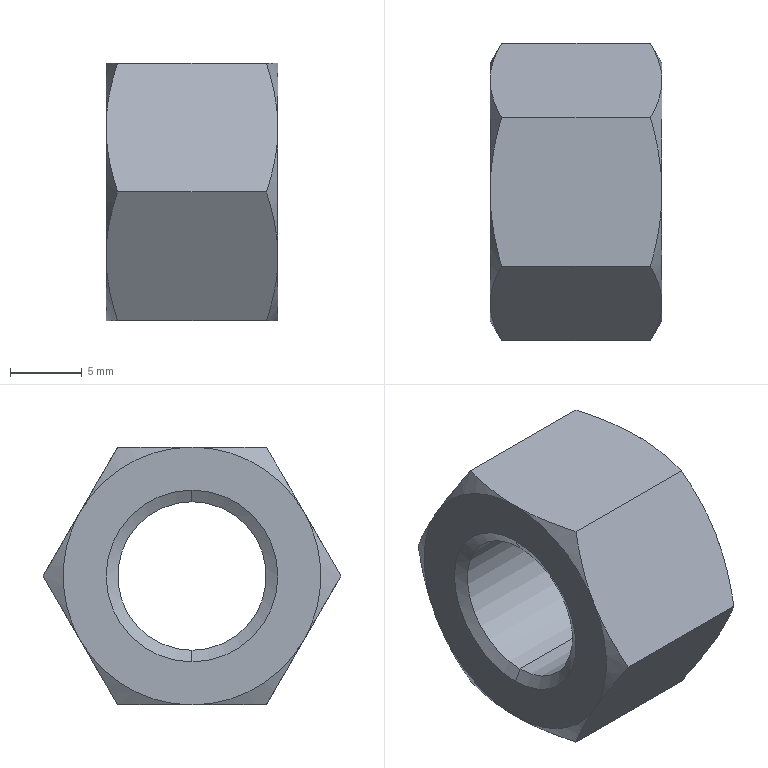Part | SolidWorks | features BaseBody 1 | 1 solid | 26 faces | box 12 x 20.785 x 18 mm | volume 2327 mm3 | cone 16 | plane 8 | cylinder 2 | commonest cylinder face diameters 10.376 x2
STEP:
#1=CARTESIAN_POINT('',(0.4688,0.,5.188));
#2=VERTEX_POINT('',#1);
#3=CARTESIAN_POINT('',(0.4688,0.,-5.188));
#4=VERTEX_POINT('',#3);
#5=CARTESIAN_POINT('',(0.4688,0.,0.));
#6=DIRECTION('',(1.,0.,0.));
#7=DIRECTION('',(0.,0.,-1.));
#8=AXIS2_PLACEMENT_3D('',#5,#6,#7);
#9=CIRCLE('',#8,5.188);
#10=EDGE_CURVE('',#2,#4,#9,.T.);
#11=ORIENTED_EDGE('',*,*,#10,.F.);
#12=CARTESIAN_POINT('',(11.531,0.,5.188));
#13=VERTEX_POINT('',#12);
#14=CARTESIAN_POINT('',(-18.,0.,5.188));
#15=DIRECTION('',(1.,0.,0.));
#16=VECTOR('',#15,1000.);
#17=LINE('',#14,#16);
#18=EDGE_CURVE('',#2,#13,#17,.T.);
#19=ORIENTED_EDGE('',*,*,#18,.T.);
#20=CARTESIAN_POINT('',(11.531,0.,-5.188));
#21=VERTEX_POINT('',#20);
#22=CARTESIAN_POINT('',(11.531,0.,0.));
#23=DIRECTION('',(-1.,0.,0.));
#24=DIRECTION('',(0.,0.,-1.));
#25=AXIS2_PLACEMENT_3D('',#22,#23,#24);
#26=CIRCLE('',#25,5.188);
#27=EDGE_CURVE('',#21,#13,#26,.T.);
#28=ORIENTED_EDGE('',*,*,#27,.F.);
#29=CARTESIAN_POINT('',(-18.,0.,-5.188));
#30=DIRECTION('',(1.,0.,0.));
#31=VECTOR('',#30,1000.);
#32=LINE('',#29,#31);
#33=EDGE_CURVE('',#4,#21,#32,.T.);
#34=ORIENTED_EDGE('',*,*,#33,.F.);
#35=EDGE_LOOP('',(#11,#19,#28,#34));
#36=FACE_OUTER_BOUND('',#35,.T.);
#37=CARTESIAN_POINT('',(-18.,0.,0.));
#38=DIRECTION('',(1.,0.,0.));
#39=DIRECTION('',(0.,0.,-1.));
#40=AXIS2_PLACEMENT_3D('',#37,#38,#39);
#41=CYLINDRICAL_SURFACE('',#40,5.188);
#42=ADVANCED_FACE('',(#36),#41,.F.);
#43=ORIENTED_EDGE('',*,*,#10,.T.);
#44=CARTESIAN_POINT('',(0.,0.,-6.));
#45=VERTEX_POINT('',#44);
#46=CARTESIAN_POINT('',(0.,0.,-6.));
#47=DIRECTION('',(-0.5,0.,-0.866));
#48=VECTOR('',#47,1000.);
#49=LINE('',#46,#48);
#50=EDGE_CURVE('',#4,#45,#49,.T.);
#51=ORIENTED_EDGE('',*,*,#50,.T.);
#52=CARTESIAN_POINT('',(0.,0.,6.));
#53=VERTEX_POINT('',#52);
#54=CARTESIAN_POINT('',(0.,0.,0.));
#55=DIRECTION('',(1.,0.,0.));
#56=DIRECTION('',(0.,0.,1.));
#57=AXIS2_PLACEMENT_3D('',#54,#55,#56);
#58=CIRCLE('',#57,6.);
#59=EDGE_CURVE('',#53,#45,#58,.T.);
#60=ORIENTED_EDGE('',*,*,#59,.F.);
#61=CARTESIAN_POINT('',(0.,0.,6.));
#62=DIRECTION('',(-0.5,0.,0.866));
#63=VECTOR('',#62,1000.);
#64=LINE('',#61,#63);
#65=EDGE_CURVE('',#2,#53,#64,.T.);
#66=ORIENTED_EDGE('',*,*,#65,.F.);
#67=EDGE_LOOP('',(#43,#51,#60,#66));
#68=FACE_OUTER_BOUND('',#67,.T.);
#69=CARTESIAN_POINT('',(0.,0.,0.));
#70=DIRECTION('',(-1.,0.,0.));
#71=DIRECTION('',(0.,0.,1.));
#72=AXIS2_PLACEMENT_3D('',#69,#70,#71);
#73=CONICAL_SURFACE('',#72,6.,1.047);
#74=ADVANCED_FACE('',(#68),#73,.F.);
#75=ORIENTED_EDGE('',*,*,#27,.T.);
#76=CARTESIAN_POINT('',(12.,0.,6.));
#77=VERTEX_POINT('',#76);
#78=CARTESIAN_POINT('',(12.,0.,6.));
#79=DIRECTION('',(0.5,0.,0.866));
#80=VECTOR('',#79,1000.);
#81=LINE('',#78,#80);
#82=EDGE_CURVE('',#13,#77,#81,.T.);
#83=ORIENTED_EDGE('',*,*,#82,.T.);
#84=CARTESIAN_POINT('',(12.,0.,-6.));
#85=VERTEX_POINT('',#84);
#86=CARTESIAN_POINT('',(12.,0.,0.));
#87=DIRECTION('',(-1.,0.,0.));
#88=DIRECTION('',(0.,0.,-1.));
#89=AXIS2_PLACEMENT_3D('',#86,#87,#88);
#90=CIRCLE('',#89,6.);
#91=EDGE_CURVE('',#85,#77,#90,.T.);
#92=ORIENTED_EDGE('',*,*,#91,.F.);
#93=CARTESIAN_POINT('',(12.,0.,-6.));
#94=DIRECTION('',(0.5,0.,-0.866));
#95=VECTOR('',#94,1000.);
#96=LINE('',#93,#95);
#97=EDGE_CURVE('',#21,#85,#96,.T.);
#98=ORIENTED_EDGE('',*,*,#97,.F.);
#99=EDGE_LOOP('',(#75,#83,#92,#98));
#100=FACE_OUTER_BOUND('',#99,.T.);
#101=CARTESIAN_POINT('',(12.,0.,0.));
#102=DIRECTION('',(1.,0.,0.));
#103=DIRECTION('',(0.,0.,-1.));
#104=AXIS2_PLACEMENT_3D('',#101,#102,#103);
#105=CONICAL_SURFACE('',#104,6.,1.047);
#106=ADVANCED_FACE('',(#100),#105,.F.);
#107=ORIENTED_EDGE('',*,*,#18,.F.);
#108=CARTESIAN_POINT('',(0.4688,0.,0.));
#109=DIRECTION('',(1.,0.,0.));
#110=DIRECTION('',(0.,0.,-1.));
#111=AXIS2_PLACEMENT_3D('',#108,#109,#110);
#112=CIRCLE('',#111,5.188);
#113=EDGE_CURVE('',#4,#2,#112,.T.);
#114=ORIENTED_EDGE('',*,*,#113,.F.);
#115=ORIENTED_EDGE('',*,*,#33,.T.);
#116=CARTESIAN_POINT('',(11.531,0.,0.));
#117=DIRECTION('',(-1.,0.,0.));
#118=DIRECTION('',(0.,0.,-1.));
#119=AXIS2_PLACEMENT_3D('',#116,#117,#118);
#120=CIRCLE('',#119,5.188);
#121=EDGE_CURVE('',#13,#21,#120,.T.);
#122=ORIENTED_EDGE('',*,*,#121,.F.);
#123=EDGE_LOOP('',(#107,#114,#115,#122));
#124=FACE_OUTER_BOUND('',#123,.T.);
#125=CARTESIAN_POINT('',(-18.,0.,0.));
#126=DIRECTION('',(1.,0.,0.));
#127=DIRECTION('',(0.,0.,-1.));
#128=AXIS2_PLACEMENT_3D('',#125,#126,#127);
#129=CYLINDRICAL_SURFACE('',#128,5.188);
#130=ADVANCED_FACE('',(#124),#129,.F.);
#131=ORIENTED_EDGE('',*,*,#50,.F.);
#132=ORIENTED_EDGE('',*,*,#113,.T.);
#133=ORIENTED_EDGE('',*,*,#65,.T.);
#134=CARTESIAN_POINT('',(0.,0.,0.));
#135=DIRECTION('',(1.,0.,0.));
#136=DIRECTION('',(0.,0.,1.));
#137=AXIS2_PLACEMENT_3D('',#134,#135,#136);
#138=CIRCLE('',#137,6.);
#139=EDGE_CURVE('',#45,#53,#138,.T.);
#140=ORIENTED_EDGE('',*,*,#139,.F.);
#141=EDGE_LOOP('',(#131,#132,#133,#140));
#142=FACE_OUTER_BOUND('',#141,.T.);
#143=CARTESIAN_POINT('',(0.,0.,0.));
#144=DIRECTION('',(-1.,0.,0.));
#145=DIRECTION('',(0.,0.,1.));
#146=AXIS2_PLACEMENT_3D('',#143,#144,#145);
#147=CONICAL_SURFACE('',#146,6.,1.047);
#148=ADVANCED_FACE('',(#142),#147,.F.);
#149=ORIENTED_EDGE('',*,*,#82,.F.);
#150=ORIENTED_EDGE('',*,*,#121,.T.);
#151=ORIENTED_EDGE('',*,*,#97,.T.);
#152=CARTESIAN_POINT('',(12.,0.,0.));
#153=DIRECTION('',(-1.,0.,0.));
#154=DIRECTION('',(0.,0.,-1.));
#155=AXIS2_PLACEMENT_3D('',#152,#153,#154);
#156=CIRCLE('',#155,6.);
#157=EDGE_CURVE('',#77,#85,#156,.T.);
#158=ORIENTED_EDGE('',*,*,#157,.F.);
#159=EDGE_LOOP('',(#149,#150,#151,#158));
#160=FACE_OUTER_BOUND('',#159,.T.);
#161=CARTESIAN_POINT('',(12.,0.,0.));
#162=DIRECTION('',(1.,0.,0.));
#163=DIRECTION('',(0.,0.,-1.));
#164=AXIS2_PLACEMENT_3D('',#161,#162,#163);
#165=CONICAL_SURFACE('',#164,6.,1.047);
#166=ADVANCED_FACE('',(#160),#165,.F.);
#167=ORIENTED_EDGE('',*,*,#59,.T.);
#168=ORIENTED_EDGE('',*,*,#139,.T.);
#169=EDGE_LOOP('',(#167,#168));
#170=FACE_BOUND('',#169,.T.);
#171=CARTESIAN_POINT('',(0.,0.,9.));
#172=VERTEX_POINT('',#171);
#173=CARTESIAN_POINT('',(0.,-7.794,4.5));
#174=VERTEX_POINT('',#173);
#175=CARTESIAN_POINT('',(0.,0.,0.));
#176=DIRECTION('',(1.,0.,0.));
#177=DIRECTION('',(0.,0.,-1.));
#178=AXIS2_PLACEMENT_3D('',#175,#176,#177);
#179=CIRCLE('',#178,9.);
#180=EDGE_CURVE('',#172,#174,#179,.T.);
#181=ORIENTED_EDGE('',*,*,#180,.F.);
#182=CARTESIAN_POINT('',(0.,7.794,4.5));
#183=VERTEX_POINT('',#182);
#184=CARTESIAN_POINT('',(0.,0.,0.));
#185=DIRECTION('',(1.,0.,0.));
#186=DIRECTION('',(0.,0.,-1.));
#187=AXIS2_PLACEMENT_3D('',#184,#185,#186);
#188=CIRCLE('',#187,9.);
#189=EDGE_CURVE('',#183,#172,#188,.T.);
#190=ORIENTED_EDGE('',*,*,#189,.F.);
#191=CARTESIAN_POINT('',(0.,7.794,-4.5));
#192=VERTEX_POINT('',#191);
#193=CARTESIAN_POINT('',(0.,0.,0.));
#194=DIRECTION('',(1.,0.,0.));
#195=DIRECTION('',(0.,0.,-1.));
#196=AXIS2_PLACEMENT_3D('',#193,#194,#195);
#197=CIRCLE('',#196,9.);
#198=EDGE_CURVE('',#192,#183,#197,.T.);
#199=ORIENTED_EDGE('',*,*,#198,.F.);
#200=CARTESIAN_POINT('',(0.,0.,-9.));
#201=VERTEX_POINT('',#200);
#202=CARTESIAN_POINT('',(0.,0.,0.));
#203=DIRECTION('',(1.,0.,0.));
#204=DIRECTION('',(0.,0.,-1.));
#205=AXIS2_PLACEMENT_3D('',#202,#203,#204);
#206=CIRCLE('',#205,9.);
#207=EDGE_CURVE('',#201,#192,#206,.T.);
#208=ORIENTED_EDGE('',*,*,#207,.F.);
#209=CARTESIAN_POINT('',(0.,-7.794,-4.5));
#210=VERTEX_POINT('',#209);
#211=CARTESIAN_POINT('',(0.,0.,0.));
#212=DIRECTION('',(1.,0.,0.));
#213=DIRECTION('',(0.,0.,-1.));
#214=AXIS2_PLACEMENT_3D('',#211,#212,#213);
#215=CIRCLE('',#214,9.);
#216=EDGE_CURVE('',#210,#201,#215,.T.);
#217=ORIENTED_EDGE('',*,*,#216,.F.);
#218=CARTESIAN_POINT('',(0.,0.,0.));
#219=DIRECTION('',(1.,0.,0.));
#220=DIRECTION('',(0.,0.,-1.));
#221=AXIS2_PLACEMENT_3D('',#218,#219,#220);
#222=CIRCLE('',#221,9.);
#223=EDGE_CURVE('',#174,#210,#222,.T.);
#224=ORIENTED_EDGE('',*,*,#223,.F.);
#225=EDGE_LOOP('',(#181,#190,#199,#208,#217,#224));
#226=FACE_OUTER_BOUND('',#225,.T.);
#227=CARTESIAN_POINT('',(0.,0.,0.));
#228=DIRECTION('',(1.,0.,0.));
#229=DIRECTION('',(0.,0.,-1.));
#230=AXIS2_PLACEMENT_3D('',#227,#228,#229);
#231=PLANE('',#230);
#232=ADVANCED_FACE('',(#170,#226),#231,.F.);
#233=ORIENTED_EDGE('',*,*,#91,.T.);
#234=ORIENTED_EDGE('',*,*,#157,.T.);
#235=EDGE_LOOP('',(#233,#234));
#236=FACE_BOUND('',#235,.T.);
#237=CARTESIAN_POINT('',(12.,0.,9.));
#238=VERTEX_POINT('',#237);
#239=CARTESIAN_POINT('',(12.,-7.794,4.5));
#240=VERTEX_POINT('',#239);
#241=CARTESIAN_POINT('',(12.,0.,0.));
#242=DIRECTION('',(1.,0.,0.));
#243=DIRECTION('',(0.,0.,1.));
#244=AXIS2_PLACEMENT_3D('',#241,#242,#243);
#245=CIRCLE('',#244,9.);
#246=EDGE_CURVE('',#238,#240,#245,.T.);
#247=ORIENTED_EDGE('',*,*,#246,.T.);
#248=CARTESIAN_POINT('',(12.,-7.794,-4.5));
#249=VERTEX_POINT('',#248);
#250=CARTESIAN_POINT('',(12.,0.,0.));
#251=DIRECTION('',(1.,0.,0.));
#252=DIRECTION('',(0.,0.,1.));
#253=AXIS2_PLACEMENT_3D('',#250,#251,#252);
#254=CIRCLE('',#253,9.);
#255=EDGE_CURVE('',#240,#249,#254,.T.);
#256=ORIENTED_EDGE('',*,*,#255,.T.);
#257=CARTESIAN_POINT('',(12.,0.,-9.));
#258=VERTEX_POINT('',#257);
#259=CARTESIAN_POINT('',(12.,0.,0.));
#260=DIRECTION('',(1.,0.,0.));
#261=DIRECTION('',(0.,0.,1.));
#262=AXIS2_PLACEMENT_3D('',#259,#260,#261);
#263=CIRCLE('',#262,9.);
#264=EDGE_CURVE('',#249,#258,#263,.T.);
#265=ORIENTED_EDGE('',*,*,#264,.T.);
#266=CARTESIAN_POINT('',(12.,7.794,-4.5));
#267=VERTEX_POINT('',#266);
#268=CARTESIAN_POINT('',(12.,0.,0.));
#269=DIRECTION('',(1.,0.,0.));
#270=DIRECTION('',(0.,0.,1.));
#271=AXIS2_PLACEMENT_3D('',#268,#269,#270);
#272=CIRCLE('',#271,9.);
#273=EDGE_CURVE('',#258,#267,#272,.T.);
#274=ORIENTED_EDGE('',*,*,#273,.T.);
#275=CARTESIAN_POINT('',(12.,7.794,4.5));
#276=VERTEX_POINT('',#275);
#277=CARTESIAN_POINT('',(12.,0.,0.));
#278=DIRECTION('',(1.,0.,0.));
#279=DIRECTION('',(0.,0.,1.));
#280=AXIS2_PLACEMENT_3D('',#277,#278,#279);
#281=CIRCLE('',#280,9.);
#282=EDGE_CURVE('',#267,#276,#281,.T.);
#283=ORIENTED_EDGE('',*,*,#282,.T.);
#284=CARTESIAN_POINT('',(12.,0.,0.));
#285=DIRECTION('',(1.,0.,0.));
#286=DIRECTION('',(0.,0.,1.));
#287=AXIS2_PLACEMENT_3D('',#284,#285,#286);
#288=CIRCLE('',#287,9.);
#289=EDGE_CURVE('',#276,#238,#288,.T.);
#290=ORIENTED_EDGE('',*,*,#289,.T.);
#291=EDGE_LOOP('',(#247,#256,#265,#274,#283,#290));
#292=FACE_OUTER_BOUND('',#291,.T.);
#293=CARTESIAN_POINT('',(12.,0.,0.));
#294=DIRECTION('',(1.,0.,0.));
#295=DIRECTION('',(0.,0.,-1.));
#296=AXIS2_PLACEMENT_3D('',#293,#294,#295);
#297=PLANE('',#296);
#298=ADVANCED_FACE('',(#236,#292),#297,.T.);
#299=ORIENTED_EDGE('',*,*,#223,.T.);
#300=CARTESIAN_POINT('',(0.8038,-10.392,0.000000014));
#301=VERTEX_POINT('',#300);
#302=CARTESIAN_POINT('',(0.,-7.794,-4.5));
#303=CARTESIAN_POINT('',(0.,-8.238,-3.732));
#304=CARTESIAN_POINT('',(0.07685,-8.675,-2.974));
#305=CARTESIAN_POINT('',(0.3567,-9.54,-1.476));
#306=CARTESIAN_POINT('',(0.5588,-9.968,-0.7351));
#307=CARTESIAN_POINT('',(0.8038,-10.392,0.000000014));
#308=B_SPLINE_CURVE_WITH_KNOTS('',3,(#302,#303,#304,#305,#306,#307),.UNSPECIFIED.,.F.,.F.,(4,2,4),(0.,0.002629,0.005258),.UNSPECIFIED.);
#309=EDGE_CURVE('',#210,#301,#308,.T.);
#310=ORIENTED_EDGE('',*,*,#309,.T.);
#311=CARTESIAN_POINT('',(0.8038,-10.392,0.000000014));
#312=CARTESIAN_POINT('',(0.5588,-9.968,0.7351));
#313=CARTESIAN_POINT('',(0.3567,-9.54,1.476));
#314=CARTESIAN_POINT('',(0.07685,-8.675,2.974));
#315=CARTESIAN_POINT('',(0.,-8.238,3.732));
#316=CARTESIAN_POINT('',(0.,-7.794,4.5));
#317=B_SPLINE_CURVE_WITH_KNOTS('',3,(#311,#312,#313,#314,#315,#316),.UNSPECIFIED.,.F.,.F.,(4,2,4),(0.,0.002629,0.005258),.UNSPECIFIED.);
#318=EDGE_CURVE('',#301,#174,#317,.T.);
#319=ORIENTED_EDGE('',*,*,#318,.T.);
#320=EDGE_LOOP('',(#299,#310,#319));
#321=FACE_OUTER_BOUND('',#320,.T.);
#322=CARTESIAN_POINT('',(0.8087,0.,0.));
#323=DIRECTION('',(1.,0.,0.));
#324=DIRECTION('',(0.,0.,-1.));
#325=AXIS2_PLACEMENT_3D('',#322,#323,#324);
#326=CONICAL_SURFACE('',#325,10.401,1.047);
#327=ADVANCED_FACE('',(#321),#326,.T.);
#328=ORIENTED_EDGE('',*,*,#180,.T.);
#329=CARTESIAN_POINT('',(0.8038,-5.196,9.));
#330=VERTEX_POINT('',#329);
#331=CARTESIAN_POINT('',(0.,-7.794,4.5));
#332=CARTESIAN_POINT('',(0.,-7.351,5.268));
#333=CARTESIAN_POINT('',(0.07685,-6.913,6.026));
#334=CARTESIAN_POINT('',(0.3567,-6.048,7.524));
#335=CARTESIAN_POINT('',(0.5588,-5.621,8.265));
#336=CARTESIAN_POINT('',(0.8038,-5.196,9.));
#337=B_SPLINE_CURVE_WITH_KNOTS('',3,(#331,#332,#333,#334,#335,#336),.UNSPECIFIED.,.F.,.F.,(4,2,4),(0.,0.002629,0.005258),.UNSPECIFIED.);
#338=EDGE_CURVE('',#174,#330,#337,.T.);
#339=ORIENTED_EDGE('',*,*,#338,.T.);
#340=CARTESIAN_POINT('',(0.8038,-5.196,9.));
#341=CARTESIAN_POINT('',(0.5588,-4.347,9.));
#342=CARTESIAN_POINT('',(0.3567,-3.492,9.));
#343=CARTESIAN_POINT('',(0.07685,-1.762,9.));
#344=CARTESIAN_POINT('',(0.,-0.8868,9.));
#345=CARTESIAN_POINT('',(0.,0.,9.));
#346=B_SPLINE_CURVE_WITH_KNOTS('',3,(#340,#341,#342,#343,#344,#345),.UNSPECIFIED.,.F.,.F.,(4,2,4),(0.,0.002629,0.005258),.UNSPECIFIED.);
#347=EDGE_CURVE('',#330,#172,#346,.T.);
#348=ORIENTED_EDGE('',*,*,#347,.T.);
#349=EDGE_LOOP('',(#328,#339,#348));
#350=FACE_OUTER_BOUND('',#349,.T.);
#351=CARTESIAN_POINT('',(0.8087,0.,0.));
#352=DIRECTION('',(1.,0.,0.));
#353=DIRECTION('',(0.,0.,-1.));
#354=AXIS2_PLACEMENT_3D('',#351,#352,#353);
#355=CONICAL_SURFACE('',#354,10.401,1.047);
#356=ADVANCED_FACE('',(#350),#355,.T.);
#357=ORIENTED_EDGE('',*,*,#189,.T.);
#358=CARTESIAN_POINT('',(0.8038,5.196,9.));
#359=VERTEX_POINT('',#358);
#360=CARTESIAN_POINT('',(0.,0.,9.));
#361=CARTESIAN_POINT('',(0.,0.8868,9.));
#362=CARTESIAN_POINT('',(0.07685,1.762,9.));
#363=CARTESIAN_POINT('',(0.3567,3.492,9.));
#364=CARTESIAN_POINT('',(0.5588,4.347,9.));
#365=CARTESIAN_POINT('',(0.8038,5.196,9.));
#366=B_SPLINE_CURVE_WITH_KNOTS('',3,(#360,#361,#362,#363,#364,#365),.UNSPECIFIED.,.F.,.F.,(4,2,4),(0.,0.002629,0.005258),.UNSPECIFIED.);
#367=EDGE_CURVE('',#172,#359,#366,.T.);
#368=ORIENTED_EDGE('',*,*,#367,.T.);
#369=CARTESIAN_POINT('',(0.8038,5.196,9.));
#370=CARTESIAN_POINT('',(0.5588,5.621,8.265));
#371=CARTESIAN_POINT('',(0.3567,6.048,7.524));
#372=CARTESIAN_POINT('',(0.07685,6.913,6.026));
#373=CARTESIAN_POINT('',(0.,7.351,5.268));
#374=CARTESIAN_POINT('',(0.,7.794,4.5));
#375=B_SPLINE_CURVE_WITH_KNOTS('',3,(#369,#370,#371,#372,#373,#374),.UNSPECIFIED.,.F.,.F.,(4,2,4),(0.,0.002629,0.005258),.UNSPECIFIED.);
#376=EDGE_CURVE('',#359,#183,#375,.T.);
#377=ORIENTED_EDGE('',*,*,#376,.T.);
#378=EDGE_LOOP('',(#357,#368,#377));
#379=FACE_OUTER_BOUND('',#378,.T.);
#380=CARTESIAN_POINT('',(0.8087,0.,0.));
#381=DIRECTION('',(1.,0.,0.));
#382=DIRECTION('',(0.,0.,-1.));
#383=AXIS2_PLACEMENT_3D('',#380,#381,#382);
#384=CONICAL_SURFACE('',#383,10.401,1.047);
#385=ADVANCED_FACE('',(#379),#384,.T.);
#386=ORIENTED_EDGE('',*,*,#198,.T.);
#387=CARTESIAN_POINT('',(0.8038,10.392,-0.000000014));
#388=VERTEX_POINT('',#387);
#389=CARTESIAN_POINT('',(0.,7.794,4.5));
#390=CARTESIAN_POINT('',(0.,8.238,3.732));
#391=CARTESIAN_POINT('',(0.07685,8.675,2.974));
#392=CARTESIAN_POINT('',(0.3567,9.54,1.476));
#393=CARTESIAN_POINT('',(0.5588,9.968,0.7351));
#394=CARTESIAN_POINT('',(0.8038,10.392,-0.000000014));
#395=B_SPLINE_CURVE_WITH_KNOTS('',3,(#389,#390,#391,#392,#393,#394),.UNSPECIFIED.,.F.,.F.,(4,2,4),(0.,0.002629,0.005258),.UNSPECIFIED.);
#396=EDGE_CURVE('',#183,#388,#395,.T.);
#397=ORIENTED_EDGE('',*,*,#396,.T.);
#398=CARTESIAN_POINT('',(0.8038,10.392,-0.000000014));
#399=CARTESIAN_POINT('',(0.5588,9.968,-0.7351));
#400=CARTESIAN_POINT('',(0.3567,9.54,-1.476));
#401=CARTESIAN_POINT('',(0.07685,8.675,-2.974));
#402=CARTESIAN_POINT('',(0.,8.238,-3.732));
#403=CARTESIAN_POINT('',(0.,7.794,-4.5));
#404=B_SPLINE_CURVE_WITH_KNOTS('',3,(#398,#399,#400,#401,#402,#403),.UNSPECIFIED.,.F.,.F.,(4,2,4),(0.,0.002629,0.005258),.UNSPECIFIED.);
#405=EDGE_CURVE('',#388,#192,#404,.T.);
#406=ORIENTED_EDGE('',*,*,#405,.T.);
#407=EDGE_LOOP('',(#386,#397,#406));
#408=FACE_OUTER_BOUND('',#407,.T.);
#409=CARTESIAN_POINT('',(0.8087,0.,0.));
#410=DIRECTION('',(1.,0.,0.));
#411=DIRECTION('',(0.,0.,-1.));
#412=AXIS2_PLACEMENT_3D('',#409,#410,#411);
#413=CONICAL_SURFACE('',#412,10.401,1.047);
#414=ADVANCED_FACE('',(#408),#413,.T.);
#415=CARTESIAN_POINT('',(0.8038,5.196,-9.));
#416=VERTEX_POINT('',#415);
#417=CARTESIAN_POINT('',(0.8038,5.196,-9.));
#418=CARTESIAN_POINT('',(0.5588,4.347,-9.));
#419=CARTESIAN_POINT('',(0.3567,3.492,-9.));
#420=CARTESIAN_POINT('',(0.07685,1.762,-9.));
#421=CARTESIAN_POINT('',(0.,0.8868,-9.));
#422=CARTESIAN_POINT('',(0.,0.,-9.));
#423=B_SPLINE_CURVE_WITH_KNOTS('',3,(#417,#418,#419,#420,#421,#422),.UNSPECIFIED.,.F.,.F.,(4,2,4),(0.,0.002629,0.005258),.UNSPECIFIED.);
#424=EDGE_CURVE('',#416,#201,#423,.T.);
#425=ORIENTED_EDGE('',*,*,#424,.T.);
#426=ORIENTED_EDGE('',*,*,#207,.T.);
#427=CARTESIAN_POINT('',(0.,7.794,-4.5));
#428=CARTESIAN_POINT('',(0.,7.351,-5.268));
#429=CARTESIAN_POINT('',(0.07685,6.913,-6.026));
#430=CARTESIAN_POINT('',(0.3567,6.048,-7.524));
#431=CARTESIAN_POINT('',(0.5588,5.621,-8.265));
#432=CARTESIAN_POINT('',(0.8038,5.196,-9.));
#433=B_SPLINE_CURVE_WITH_KNOTS('',3,(#427,#428,#429,#430,#431,#432),.UNSPECIFIED.,.F.,.F.,(4,2,4),(0.,0.002629,0.005258),.UNSPECIFIED.);
#434=EDGE_CURVE('',#192,#416,#433,.T.);
#435=ORIENTED_EDGE('',*,*,#434,.T.);
#436=EDGE_LOOP('',(#425,#426,#435));
#437=FACE_OUTER_BOUND('',#436,.T.);
#438=CARTESIAN_POINT('',(0.8087,0.,0.));
#439=DIRECTION('',(1.,0.,0.));
#440=DIRECTION('',(0.,0.,-1.));
#441=AXIS2_PLACEMENT_3D('',#438,#439,#440);
#442=CONICAL_SURFACE('',#441,10.401,1.047);
#443=ADVANCED_FACE('',(#437),#442,.T.);
#444=CARTESIAN_POINT('',(0.8038,-5.196,-9.));
#445=VERTEX_POINT('',#444);
#446=CARTESIAN_POINT('',(0.8038,-5.196,-9.));
#447=CARTESIAN_POINT('',(0.5588,-5.621,-8.265));
#448=CARTESIAN_POINT('',(0.3567,-6.048,-7.524));
#449=CARTESIAN_POINT('',(0.07685,-6.913,-6.026));
#450=CARTESIAN_POINT('',(0.,-7.351,-5.268));
#451=CARTESIAN_POINT('',(0.,-7.794,-4.5));
#452=B_SPLINE_CURVE_WITH_KNOTS('',3,(#446,#447,#448,#449,#450,#451),.UNSPECIFIED.,.F.,.F.,(4,2,4),(0.,0.002629,0.005258),.UNSPECIFIED.);
#453=EDGE_CURVE('',#445,#210,#452,.T.);
#454=ORIENTED_EDGE('',*,*,#453,.T.);
#455=ORIENTED_EDGE('',*,*,#216,.T.);
#456=CARTESIAN_POINT('',(0.,0.,-9.));
#457=CARTESIAN_POINT('',(0.,-0.8868,-9.));
#458=CARTESIAN_POINT('',(0.07685,-1.762,-9.));
#459=CARTESIAN_POINT('',(0.3567,-3.492,-9.));
#460=CARTESIAN_POINT('',(0.5588,-4.347,-9.));
#461=CARTESIAN_POINT('',(0.8038,-5.196,-9.));
#462=B_SPLINE_CURVE_WITH_KNOTS('',3,(#456,#457,#458,#459,#460,#461),.UNSPECIFIED.,.F.,.F.,(4,2,4),(0.,0.002629,0.005258),.UNSPECIFIED.);
#463=EDGE_CURVE('',#201,#445,#462,.T.);
#464=ORIENTED_EDGE('',*,*,#463,.T.);
#465=EDGE_LOOP('',(#454,#455,#464));
#466=FACE_OUTER_BOUND('',#465,.T.);
#467=CARTESIAN_POINT('',(0.8087,0.,0.));
#468=DIRECTION('',(1.,0.,0.));
#469=DIRECTION('',(0.,0.,-1.));
#470=AXIS2_PLACEMENT_3D('',#467,#468,#469);
#471=CONICAL_SURFACE('',#470,10.401,1.047);
#472=ADVANCED_FACE('',(#466),#471,.T.);
#473=CARTESIAN_POINT('',(11.196,-10.392,0.000000038));
#474=VERTEX_POINT('',#473);
#475=CARTESIAN_POINT('',(11.196,-10.392,0.000000038));
#476=CARTESIAN_POINT('',(11.441,-9.968,-0.7351));
#477=CARTESIAN_POINT('',(11.643,-9.54,-1.476));
#478=CARTESIAN_POINT('',(11.923,-8.675,-2.974));
#479=CARTESIAN_POINT('',(12.,-8.238,-3.732));
#480=CARTESIAN_POINT('',(12.,-7.794,-4.5));
#481=B_SPLINE_CURVE_WITH_KNOTS('',3,(#475,#476,#477,#478,#479,#480),.UNSPECIFIED.,.F.,.F.,(4,2,4),(0.,0.002629,0.005258),.UNSPECIFIED.);
#482=EDGE_CURVE('',#474,#249,#481,.T.);
#483=ORIENTED_EDGE('',*,*,#482,.T.);
#484=ORIENTED_EDGE('',*,*,#255,.F.);
#485=CARTESIAN_POINT('',(12.,-7.794,4.5));
#486=CARTESIAN_POINT('',(12.,-8.238,3.732));
#487=CARTESIAN_POINT('',(11.923,-8.675,2.974));
#488=CARTESIAN_POINT('',(11.643,-9.54,1.476));
#489=CARTESIAN_POINT('',(11.441,-9.968,0.7351));
#490=CARTESIAN_POINT('',(11.196,-10.392,0.000000038));
#491=B_SPLINE_CURVE_WITH_KNOTS('',3,(#485,#486,#487,#488,#489,#490),.UNSPECIFIED.,.F.,.F.,(4,2,4),(0.,0.002629,0.005258),.UNSPECIFIED.);
#492=EDGE_CURVE('',#240,#474,#491,.T.);
#493=ORIENTED_EDGE('',*,*,#492,.T.);
#494=EDGE_LOOP('',(#483,#484,#493));
#495=FACE_OUTER_BOUND('',#494,.T.);
#496=CARTESIAN_POINT('',(11.191,0.,0.));
#497=DIRECTION('',(-1.,0.,0.));
#498=DIRECTION('',(0.,0.,1.));
#499=AXIS2_PLACEMENT_3D('',#496,#497,#498);
#500=CONICAL_SURFACE('',#499,10.401,1.047);
#501=ADVANCED_FACE('',(#495),#500,.T.);
#502=CARTESIAN_POINT('',(11.196,-5.196,9.));
#503=VERTEX_POINT('',#502);
#504=CARTESIAN_POINT('',(11.196,-5.196,9.));
#505=CARTESIAN_POINT('',(11.441,-5.621,8.265));
#506=CARTESIAN_POINT('',(11.643,-6.048,7.524));
#507=CARTESIAN_POINT('',(11.923,-6.913,6.026));
#508=CARTESIAN_POINT('',(12.,-7.351,5.268));
#509=CARTESIAN_POINT('',(12.,-7.794,4.5));
#510=B_SPLINE_CURVE_WITH_KNOTS('',3,(#504,#505,#506,#507,#508,#509),.UNSPECIFIED.,.F.,.F.,(4,2,4),(0.,0.002629,0.005258),.UNSPECIFIED.);
#511=EDGE_CURVE('',#503,#240,#510,.T.);
#512=ORIENTED_EDGE('',*,*,#511,.T.);
#513=ORIENTED_EDGE('',*,*,#246,.F.);
#514=CARTESIAN_POINT('',(12.,0.,9.));
#515=CARTESIAN_POINT('',(12.,-0.8868,9.));
#516=CARTESIAN_POINT('',(11.923,-1.762,9.));
#517=CARTESIAN_POINT('',(11.643,-3.492,9.));
#518=CARTESIAN_POINT('',(11.441,-4.347,9.));
#519=CARTESIAN_POINT('',(11.196,-5.196,9.));
#520=B_SPLINE_CURVE_WITH_KNOTS('',3,(#514,#515,#516,#517,#518,#519),.UNSPECIFIED.,.F.,.F.,(4,2,4),(0.,0.002629,0.005258),.UNSPECIFIED.);
#521=EDGE_CURVE('',#238,#503,#520,.T.);
#522=ORIENTED_EDGE('',*,*,#521,.T.);
#523=EDGE_LOOP('',(#512,#513,#522));
#524=FACE_OUTER_BOUND('',#523,.T.);
#525=CARTESIAN_POINT('',(11.191,0.,0.));
#526=DIRECTION('',(-1.,0.,0.));
#527=DIRECTION('',(0.,0.,1.));
#528=AXIS2_PLACEMENT_3D('',#525,#526,#527);
#529=CONICAL_SURFACE('',#528,10.401,1.047);
#530=ADVANCED_FACE('',(#524),#529,.T.);
#531=CARTESIAN_POINT('',(11.196,5.196,9.));
#532=VERTEX_POINT('',#531);
#533=CARTESIAN_POINT('',(11.196,5.196,9.));
#534=CARTESIAN_POINT('',(11.441,4.347,9.));
#535=CARTESIAN_POINT('',(11.643,3.492,9.));
#536=CARTESIAN_POINT('',(11.923,1.762,9.));
#537=CARTESIAN_POINT('',(12.,0.8868,9.));
#538=CARTESIAN_POINT('',(12.,0.,9.));
#539=B_SPLINE_CURVE_WITH_KNOTS('',3,(#533,#534,#535,#536,#537,#538),.UNSPECIFIED.,.F.,.F.,(4,2,4),(0.,0.002629,0.005258),.UNSPECIFIED.);
#540=EDGE_CURVE('',#532,#238,#539,.T.);
#541=ORIENTED_EDGE('',*,*,#540,.T.);
#542=ORIENTED_EDGE('',*,*,#289,.F.);
#543=CARTESIAN_POINT('',(12.,7.794,4.5));
#544=CARTESIAN_POINT('',(12.,7.351,5.268));
#545=CARTESIAN_POINT('',(11.923,6.913,6.026));
#546=CARTESIAN_POINT('',(11.643,6.048,7.524));
#547=CARTESIAN_POINT('',(11.441,5.621,8.265));
#548=CARTESIAN_POINT('',(11.196,5.196,9.));
#549=B_SPLINE_CURVE_WITH_KNOTS('',3,(#543,#544,#545,#546,#547,#548),.UNSPECIFIED.,.F.,.F.,(4,2,4),(0.,0.002629,0.005258),.UNSPECIFIED.);
#550=EDGE_CURVE('',#276,#532,#549,.T.);
#551=ORIENTED_EDGE('',*,*,#550,.T.);
#552=EDGE_LOOP('',(#541,#542,#551));
#553=FACE_OUTER_BOUND('',#552,.T.);
#554=CARTESIAN_POINT('',(11.191,0.,0.));
#555=DIRECTION('',(-1.,0.,0.));
#556=DIRECTION('',(0.,0.,1.));
#557=AXIS2_PLACEMENT_3D('',#554,#555,#556);
#558=CONICAL_SURFACE('',#557,10.401,1.047);
#559=ADVANCED_FACE('',(#553),#558,.T.);
#560=ORIENTED_EDGE('',*,*,#282,.F.);
#561=CARTESIAN_POINT('',(11.196,10.392,0.000000014));
#562=VERTEX_POINT('',#561);
#563=CARTESIAN_POINT('',(12.,7.794,-4.5));
#564=CARTESIAN_POINT('',(12.,8.238,-3.732));
#565=CARTESIAN_POINT('',(11.923,8.675,-2.974));
#566=CARTESIAN_POINT('',(11.643,9.54,-1.476));
#567=CARTESIAN_POINT('',(11.441,9.968,-0.7351));
#568=CARTESIAN_POINT('',(11.196,10.392,0.000000014));
#569=B_SPLINE_CURVE_WITH_KNOTS('',3,(#563,#564,#565,#566,#567,#568),.UNSPECIFIED.,.F.,.F.,(4,2,4),(0.,0.002629,0.005258),.UNSPECIFIED.);
#570=EDGE_CURVE('',#267,#562,#569,.T.);
#571=ORIENTED_EDGE('',*,*,#570,.T.);
#572=CARTESIAN_POINT('',(11.196,10.392,0.000000014));
#573=CARTESIAN_POINT('',(11.441,9.968,0.7351));
#574=CARTESIAN_POINT('',(11.643,9.54,1.476));
#575=CARTESIAN_POINT('',(11.923,8.675,2.974));
#576=CARTESIAN_POINT('',(12.,8.238,3.732));
#577=CARTESIAN_POINT('',(12.,7.794,4.5));
#578=B_SPLINE_CURVE_WITH_KNOTS('',3,(#572,#573,#574,#575,#576,#577),.UNSPECIFIED.,.F.,.F.,(4,2,4),(0.,0.002629,0.005258),.UNSPECIFIED.);
#579=EDGE_CURVE('',#562,#276,#578,.T.);
#580=ORIENTED_EDGE('',*,*,#579,.T.);
#581=EDGE_LOOP('',(#560,#571,#580));
#582=FACE_OUTER_BOUND('',#581,.T.);
#583=CARTESIAN_POINT('',(11.191,0.,0.));
#584=DIRECTION('',(-1.,0.,0.));
#585=DIRECTION('',(0.,0.,1.));
#586=AXIS2_PLACEMENT_3D('',#583,#584,#585);
#587=CONICAL_SURFACE('',#586,10.401,1.047);
#588=ADVANCED_FACE('',(#582),#587,.T.);
#589=ORIENTED_EDGE('',*,*,#273,.F.);
#590=CARTESIAN_POINT('',(11.196,5.196,-9.));
#591=VERTEX_POINT('',#590);
#592=CARTESIAN_POINT('',(12.,0.,-9.));
#593=CARTESIAN_POINT('',(12.,0.8868,-9.));
#594=CARTESIAN_POINT('',(11.923,1.762,-9.));
#595=CARTESIAN_POINT('',(11.643,3.492,-9.));
#596=CARTESIAN_POINT('',(11.441,4.347,-9.));
#597=CARTESIAN_POINT('',(11.196,5.196,-9.));
#598=B_SPLINE_CURVE_WITH_KNOTS('',3,(#592,#593,#594,#595,#596,#597),.UNSPECIFIED.,.F.,.F.,(4,2,4),(0.,0.002629,0.005258),.UNSPECIFIED.);
#599=EDGE_CURVE('',#258,#591,#598,.T.);
#600=ORIENTED_EDGE('',*,*,#599,.T.);
#601=CARTESIAN_POINT('',(11.196,5.196,-9.));
#602=CARTESIAN_POINT('',(11.441,5.621,-8.265));
#603=CARTESIAN_POINT('',(11.643,6.048,-7.524));
#604=CARTESIAN_POINT('',(11.923,6.913,-6.026));
#605=CARTESIAN_POINT('',(12.,7.351,-5.268));
#606=CARTESIAN_POINT('',(12.,7.794,-4.5));
#607=B_SPLINE_CURVE_WITH_KNOTS('',3,(#601,#602,#603,#604,#605,#606),.UNSPECIFIED.,.F.,.F.,(4,2,4),(0.,0.002629,0.005258),.UNSPECIFIED.);
#608=EDGE_CURVE('',#591,#267,#607,.T.);
#609=ORIENTED_EDGE('',*,*,#608,.T.);
#610=EDGE_LOOP('',(#589,#600,#609));
#611=FACE_OUTER_BOUND('',#610,.T.);
#612=CARTESIAN_POINT('',(11.191,0.,0.));
#613=DIRECTION('',(-1.,0.,0.));
#614=DIRECTION('',(0.,0.,1.));
#615=AXIS2_PLACEMENT_3D('',#612,#613,#614);
#616=CONICAL_SURFACE('',#615,10.401,1.047);
#617=ADVANCED_FACE('',(#611),#616,.T.);
#618=ORIENTED_EDGE('',*,*,#264,.F.);
#619=CARTESIAN_POINT('',(11.196,-5.196,-9.));
#620=VERTEX_POINT('',#619);
#621=CARTESIAN_POINT('',(12.,-7.794,-4.5));
#622=CARTESIAN_POINT('',(12.,-7.351,-5.268));
#623=CARTESIAN_POINT('',(11.923,-6.913,-6.026));
#624=CARTESIAN_POINT('',(11.643,-6.048,-7.524));
#625=CARTESIAN_POINT('',(11.441,-5.621,-8.265));
#626=CARTESIAN_POINT('',(11.196,-5.196,-9.));
#627=B_SPLINE_CURVE_WITH_KNOTS('',3,(#621,#622,#623,#624,#625,#626),.UNSPECIFIED.,.F.,.F.,(4,2,4),(0.,0.002629,0.005258),.UNSPECIFIED.);
#628=EDGE_CURVE('',#249,#620,#627,.T.);
#629=ORIENTED_EDGE('',*,*,#628,.T.);
#630=CARTESIAN_POINT('',(11.196,-5.196,-9.));
#631=CARTESIAN_POINT('',(11.441,-4.347,-9.));
#632=CARTESIAN_POINT('',(11.643,-3.492,-9.));
#633=CARTESIAN_POINT('',(11.923,-1.762,-9.));
#634=CARTESIAN_POINT('',(12.,-0.8868,-9.));
#635=CARTESIAN_POINT('',(12.,0.,-9.));
#636=B_SPLINE_CURVE_WITH_KNOTS('',3,(#630,#631,#632,#633,#634,#635),.UNSPECIFIED.,.F.,.F.,(4,2,4),(0.,0.002629,0.005258),.UNSPECIFIED.);
#637=EDGE_CURVE('',#620,#258,#636,.T.);
#638=ORIENTED_EDGE('',*,*,#637,.T.);
#639=EDGE_LOOP('',(#618,#629,#638));
#640=FACE_OUTER_BOUND('',#639,.T.);
#641=CARTESIAN_POINT('',(11.191,0.,0.));
#642=DIRECTION('',(-1.,0.,0.));
#643=DIRECTION('',(0.,0.,1.));
#644=AXIS2_PLACEMENT_3D('',#641,#642,#643);
#645=CONICAL_SURFACE('',#644,10.401,1.047);
#646=ADVANCED_FACE('',(#640),#645,.T.);
#647=CARTESIAN_POINT('',(0.,-10.392,0.));
#648=DIRECTION('',(-1.,0.,0.));
#649=VECTOR('',#648,1000.);
#650=LINE('',#647,#649);
#651=EDGE_CURVE('',#474,#301,#650,.T.);
#652=ORIENTED_EDGE('',*,*,#651,.T.);
#653=ORIENTED_EDGE('',*,*,#309,.F.);
#654=ORIENTED_EDGE('',*,*,#453,.F.);
#655=CARTESIAN_POINT('',(0.,-5.196,-9.));
#656=DIRECTION('',(1.,0.,0.));
#657=VECTOR('',#656,1000.);
#658=LINE('',#655,#657);
#659=EDGE_CURVE('',#445,#620,#658,.T.);
#660=ORIENTED_EDGE('',*,*,#659,.T.);
#661=ORIENTED_EDGE('',*,*,#628,.F.);
#662=ORIENTED_EDGE('',*,*,#482,.F.);
#663=EDGE_LOOP('',(#652,#653,#654,#660,#661,#662));
#664=FACE_OUTER_BOUND('',#663,.T.);
#665=CARTESIAN_POINT('',(0.,-5.196,-9.));
#666=DIRECTION('',(0.,-0.866,-0.5));
#667=DIRECTION('',(0.,0.5,-0.866));
#668=AXIS2_PLACEMENT_3D('',#665,#666,#667);
#669=PLANE('',#668);
#670=ADVANCED_FACE('',(#664),#669,.T.);
#671=ORIENTED_EDGE('',*,*,#511,.F.);
#672=CARTESIAN_POINT('',(0.,-5.196,9.));
#673=DIRECTION('',(-1.,0.,0.));
#674=VECTOR('',#673,1000.);
#675=LINE('',#672,#674);
#676=EDGE_CURVE('',#503,#330,#675,.T.);
#677=ORIENTED_EDGE('',*,*,#676,.T.);
#678=ORIENTED_EDGE('',*,*,#338,.F.);
#679=ORIENTED_EDGE('',*,*,#318,.F.);
#680=ORIENTED_EDGE('',*,*,#651,.F.);
#681=ORIENTED_EDGE('',*,*,#492,.F.);
#682=EDGE_LOOP('',(#671,#677,#678,#679,#680,#681));
#683=FACE_OUTER_BOUND('',#682,.T.);
#684=CARTESIAN_POINT('',(0.,-10.392,0.));
#685=DIRECTION('',(0.,-0.866,0.5));
#686=DIRECTION('',(0.,-0.5,-0.866));
#687=AXIS2_PLACEMENT_3D('',#684,#685,#686);
#688=PLANE('',#687);
#689=ADVANCED_FACE('',(#683),#688,.T.);
#690=ORIENTED_EDGE('',*,*,#540,.F.);
#691=CARTESIAN_POINT('',(0.,5.196,9.));
#692=DIRECTION('',(-1.,0.,0.));
#693=VECTOR('',#692,1000.);
#694=LINE('',#691,#693);
#695=EDGE_CURVE('',#532,#359,#694,.T.);
#696=ORIENTED_EDGE('',*,*,#695,.T.);
#697=ORIENTED_EDGE('',*,*,#367,.F.);
#698=ORIENTED_EDGE('',*,*,#347,.F.);
#699=ORIENTED_EDGE('',*,*,#676,.F.);
#700=ORIENTED_EDGE('',*,*,#521,.F.);
#701=EDGE_LOOP('',(#690,#696,#697,#698,#699,#700));
#702=FACE_OUTER_BOUND('',#701,.T.);
#703=CARTESIAN_POINT('',(0.,-5.196,9.));
#704=DIRECTION('',(0.,0.,1.));
#705=DIRECTION('',(1.,0.,0.));
#706=AXIS2_PLACEMENT_3D('',#703,#704,#705);
#707=PLANE('',#706);
#708=ADVANCED_FACE('',(#702),#707,.T.);
#709=ORIENTED_EDGE('',*,*,#579,.F.);
#710=CARTESIAN_POINT('',(0.,10.392,0.));
#711=DIRECTION('',(-1.,0.,0.));
#712=VECTOR('',#711,1000.);
#713=LINE('',#710,#712);
#714=EDGE_CURVE('',#562,#388,#713,.T.);
#715=ORIENTED_EDGE('',*,*,#714,.T.);
#716=ORIENTED_EDGE('',*,*,#396,.F.);
#717=ORIENTED_EDGE('',*,*,#376,.F.);
#718=ORIENTED_EDGE('',*,*,#695,.F.);
#719=ORIENTED_EDGE('',*,*,#550,.F.);
#720=EDGE_LOOP('',(#709,#715,#716,#717,#718,#719));
#721=FACE_OUTER_BOUND('',#720,.T.);
#722=CARTESIAN_POINT('',(0.,5.196,9.));
#723=DIRECTION('',(0.,0.866,0.5));
#724=DIRECTION('',(0.,-0.5,0.866));
#725=AXIS2_PLACEMENT_3D('',#722,#723,#724);
#726=PLANE('',#725);
#727=ADVANCED_FACE('',(#721),#726,.T.);
#728=CARTESIAN_POINT('',(0.,5.196,-9.));
#729=DIRECTION('',(-1.,0.,0.));
#730=VECTOR('',#729,1000.);
#731=LINE('',#728,#730);
#732=EDGE_CURVE('',#591,#416,#731,.T.);
#733=ORIENTED_EDGE('',*,*,#732,.T.);
#734=ORIENTED_EDGE('',*,*,#434,.F.);
#735=ORIENTED_EDGE('',*,*,#405,.F.);
#736=ORIENTED_EDGE('',*,*,#714,.F.);
#737=ORIENTED_EDGE('',*,*,#570,.F.);
#738=ORIENTED_EDGE('',*,*,#608,.F.);
#739=EDGE_LOOP('',(#733,#734,#735,#736,#737,#738));
#740=FACE_OUTER_BOUND('',#739,.T.);
#741=CARTESIAN_POINT('',(0.,10.392,0.));
#742=DIRECTION('',(0.,0.866,-0.5));
#743=DIRECTION('',(0.,0.5,0.866));
#744=AXIS2_PLACEMENT_3D('',#741,#742,#743);
#745=PLANE('',#744);
#746=ADVANCED_FACE('',(#740),#745,.T.);
#747=ORIENTED_EDGE('',*,*,#659,.F.);
#748=ORIENTED_EDGE('',*,*,#463,.F.);
#749=ORIENTED_EDGE('',*,*,#424,.F.);
#750=ORIENTED_EDGE('',*,*,#732,.F.);
#751=ORIENTED_EDGE('',*,*,#599,.F.);
#752=ORIENTED_EDGE('',*,*,#637,.F.);
#753=EDGE_LOOP('',(#747,#748,#749,#750,#751,#752));
#754=FACE_OUTER_BOUND('',#753,.T.);
#755=CARTESIAN_POINT('',(0.,5.196,-9.));
#756=DIRECTION('',(0.,0.,-1.));
#757=DIRECTION('',(0.,1.,0.));
#758=AXIS2_PLACEMENT_3D('',#755,#756,#757);
#759=PLANE('',#758);
#760=ADVANCED_FACE('',(#754),#759,.T.);
#761=CLOSED_SHELL('',(#42,#74,#106,#130,#148,#166,#232,#298,#327,#356,#385,#414,#443,#472,#501,#530,#559,#588,#617,#646,#670,#689,#708,#727,#746,#760));
#762=MANIFOLD_SOLID_BREP('',#761);
#763=CARTESIAN_POINT('',(0.,0.,0.));
#764=DIRECTION('',(0.,0.,1.));
#765=DIRECTION('',(1.,0.,0.));
#766=AXIS2_PLACEMENT_3D('',#763,#764,#765);
#767=(LENGTH_UNIT()NAMED_UNIT(*)SI_UNIT(.MILLI.,.METRE.));
#768=UNCERTAINTY_MEASURE_WITH_UNIT(LENGTH_MEASURE(0.00001),#767,'','');
#769=(NAMED_UNIT(*)PLANE_ANGLE_UNIT()SI_UNIT($,.RADIAN.));
#770=(NAMED_UNIT(*)SI_UNIT($,.STERADIAN.)SOLID_ANGLE_UNIT());
#771=(GEOMETRIC_REPRESENTATION_CONTEXT(3)GLOBAL_UNCERTAINTY_ASSIGNED_CONTEXT((#768))GLOBAL_UNIT_ASSIGNED_CONTEXT((#767,#769,#770))REPRESENTATION_CONTEXT('',''));
#772=ADVANCED_BREP_SHAPE_REPRESENTATION('',(#762,#766),#771);